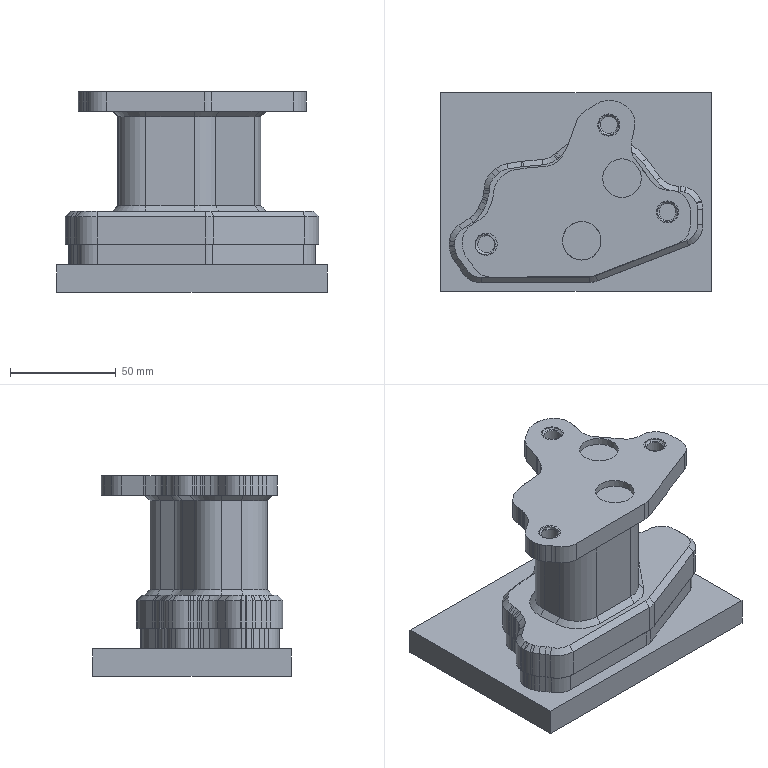NC program | NX | posted by the shop | part box 128.162 x 94.109 x 95 mm
Lines 2106 to 2518 of 2518:
2105 TOOL CALL 15 Z S8000
2106 CALL LBL101
2107 M3 M8
2108 M51
2109 CYCL DEF 32.0 TOLERANCE
2110 CYCL DEF 32.1 T0.012
2111 CYCL DEF 32.2 HSC-MODE:0
2112 L M126
2113 L A+0.0 C+0.0 FMAX
2114 L X-20.1628 Y-49.7703 FMAX
2115 L Z135. FMAX
2116 L Z72.4361 FMAX
2117 L X-17.9996 Y-44.1738 F1000.
2118 L X-55.0175 Y-29.8654
2119 CC X-49.4871 Y-15.5573
2120 C X-64.8269 Y-15.5573 DR-
2121 L Y-8.3845
2122 CC X-49.4871 Y-8.3845
2123 C X-63.8198 Y-2.9181 DR-
2124 L X-63.6526 Y-2.4797
2125 CC X-49.3199 Y-7.9461
2126 C X-53.2724 Y6.8757 DR-
2127 L X-53.2021 Y6.8944
2128 CC X-49.2496 Y-7.9274
2129 C X-49.2496 Y7.4124 DR-
2130 L X-48.4571
2131 CC X-48.4571 Y13.2602
2132 C X-43.7903 Y9.7363 DR+
2133 L X-37.044 Y18.6706
2134 CC X-11.9727 Y-.2607
2135 C X-7.4357 Y30.826 DR-
2136 L X-4.8349 Y30.4464
2137 CC X-9.3718 Y-.6402
2138 C X12.4228 Y21.9862 DR-
2139 CC X16.4797 Y26.1979
2140 C X12.9027 Y21.5717 DR+
2141 L X13.3406 Y21.2331
2142 CC X16.9177 Y25.8593
2143 C X16.4254 Y20.0323 DR+
2144 L X25.5719 Y19.2596
2145 CC X24.2807 Y3.9743
2146 C X26.5942 Y19.1386 DR-
2147 L X33.2783 Y18.1189
2148 CC X30.9648 Y2.9545
2149 C X41.0283 Y14.532 DR-
2150 L X42.9771 Y12.838
2151 CC X32.9137 Y1.2606
2152 C X48.2402 Y1.8989 DR-
2153 CC X54.0829 Y2.1423
2154 C X48.2836 Y1.3906 DR+
2155 L X48.4707 Y-.0522
2156 CC X54.2699 Y.6995
2157 C X48.6732 Y-.9956 DR+
2158 L X49.0076 Y-2.0997
2159 CC X54.6044 Y-.4047
2160 C X49.2541 Y-2.7651 DR+
2161 L X50.5606 Y-5.7266
2162 CC X55.9109 Y-3.3662
2163 C X52.7025 Y-8.2552 DR+
2164 L X57.8907 Y-11.66
2165 CC X49.4744 Y-24.4848
2166 C X64.687 Y-22.513 DR-
2167 L X64.6996 Y-22.6105
2168 CC X49.4871 Y-24.5823
2169 C X64.7942 Y-25.5824 DR-
2170 L X64.7448 Y-26.3385
2171 CC X49.4377 Y-25.3384
2172 C X63.9557 Y-30.2918 DR-
2173 L X63.5699 Y-31.4225
2174 CC X49.0519 Y-26.4691
2175 C X61.1604 Y-35.8868 DR-
2176 L X59.4035 Y-38.1457
2177 CC X64.0194 Y-41.7359
2178 C X58.7617 Y-39.176 DR+
2179 CC X44.9698 Y-32.4609
2180 C X44.905 Y-47.8006 DR-
2181 L X-6.3796 Y-47.5841
2182 CC X-6.3149 Y-32.2444
2183 C X-11.8453 Y-46.5526 DR-
2184 L X-17.9996 Y-44.1738
2185 L X-16.197 Y-39.51
2186 L X-53.2149 Y-25.2017
2187 CC X-49.4871 Y-15.5573
2188 C X-59.8269 Y-15.5573 DR-
2189 L Y-8.3845
2190 CC X-49.4871 Y-8.3845
2191 C X-59.1481 Y-4.6999 DR-
2192 L X-58.9809 Y-4.2615
2193 CC X-49.3199 Y-7.9461
2194 C X-51.984 Y2.0445 DR-
2195 CC X-49.2506 Y-7.9274
2196 C X-49.2496 Y2.4124 DR-
2197 L X-48.4571
2198 CC X-48.4571 Y13.2602
2199 C X-39.8001 Y6.7233 DR+
2200 L X-33.0538 Y15.6576
2201 CC X-11.9727 Y-.2607
2202 C X-8.1578 Y25.8784 DR-
2203 L X-5.5569 Y25.4988
2204 CC X-9.3718 Y-.6402
2205 C X8.9541 Y18.3851 DR-
2206 CC X16.4797 Y26.1979
2207 C X9.8442 Y17.6163 DR+
2208 L X10.2822 Y17.2776
2209 CC X16.9177 Y25.8593
2210 C X16.0046 Y15.05 DR+
2211 L X25.1511 Y14.2774
2212 CC X24.2807 Y3.9743
2213 C X25.8401 Y14.1958 DR-
2214 L X32.5242 Y13.1761
2215 CC X30.9648 Y2.9545
2216 C X37.7481 Y10.7583 DR-
2217 L X39.6969 Y9.0643
2218 CC X32.9137 Y1.2606
2219 C X43.2445 Y1.6908 DR-
2220 CC X54.0829 Y2.1423
2221 C X43.3251 Y.7479 DR+
2222 L X43.5123 Y-.696
2223 CC X54.2699 Y.6995
2224 C X43.8879 Y-2.4449 DR+
2225 L X44.2223 Y-3.5491
2226 CC X54.6044 Y-.4047
2227 C X44.6795 Y-4.7833 DR+
2228 L X45.9865 Y-7.7457
2229 CC X55.9109 Y-3.3662
2230 C X49.9592 Y-12.4354 DR+
2231 L X55.1474 Y-15.8402
2232 CC X49.4749 Y-24.4851
2233 C X59.7411 Y-23.2532 DR-
2234 CC X49.4871 Y-24.5823
2235 C X59.8049 Y-25.2564 DR-
2236 L X59.7555 Y-26.0125
2237 CC X49.4377 Y-25.3384
2238 C X59.2235 Y-28.6772 DR-
2239 L X58.8378 Y-29.8079
2240 CC X49.0519 Y-26.4691
2241 C X57.2136 Y-32.8171 DR-
2242 L X55.4567 Y-35.076
2243 CC X64.0194 Y-41.7359
2244 C X54.2662 Y-36.9872 DR+
2245 CC X44.9698 Y-32.4609
2246 C X44.9261 Y-42.8006 DR-
2247 L X-6.3585 Y-42.5841
2248 CC X-6.3149 Y-32.2444
2249 C X-10.0427 Y-41.8888 DR-
2250 L X-16.197 Y-39.51
2251 L X-14.3943 Y-34.8463
2252 L X-51.4122 Y-20.538
2253 CC X-49.4871 Y-15.5573
2254 C X-54.8269 Y-15.5573 DR-
2255 L Y-8.3845
2256 CC X-49.4871 Y-8.3845
2257 C X-54.4763 Y-6.4816 DR-
2258 L X-54.3091 Y-6.0433
2259 CC X-49.3199 Y-7.9461
2260 C X-50.679 Y-2.7822 DR-
2261 CC X-49.2507 Y-7.9274
2262 C X-49.2501 Y-2.5876 DR-
2263 L X-48.4571
2264 CC X-48.4571 Y13.2602
2265 C X-35.8099 Y3.7103 DR+
2266 L X-29.0636 Y12.6446
2267 CC X-11.9727 Y-.2607
2268 C X-8.8799 Y20.9308 DR-
2269 L X-6.279 Y20.5513
2270 CC X-9.3718 Y-.6402
2271 C X5.4854 Y14.784 DR-
2272 CC X16.4797 Y26.1979
2273 C X6.7858 Y13.6608 DR+
2274 L X7.2237 Y13.3221
2275 CC X16.9177 Y25.8593
2276 C X15.5837 Y10.0677 DR+
2277 L X24.7302 Y9.2951
2278 CC X24.2807 Y3.9743
2279 C X25.086 Y9.253 DR-
2280 L X31.7702 Y8.2333
2281 CC X30.9648 Y2.9545
2282 C X34.4679 Y6.9847 DR-
2283 L X36.4168 Y5.2907
2284 CC X32.9137 Y1.2606
2285 C X38.2489 Y1.4828 DR-
2286 CC X54.0829 Y2.1423
2287 C X38.3666 Y.1052 DR+
2288 L X38.5538 Y-1.3392
2289 CC X54.2699 Y.6995
2290 C X39.1025 Y-3.8942 DR+
2291 L X39.4369 Y-4.9984
2292 CC X54.6044 Y-.4047
2293 C X40.1049 Y-6.8015 DR+
2294 L X41.4121 Y-9.7643
2295 CC X55.9109 Y-3.3662
2296 C X47.2159 Y-16.6157 DR+
2297 L X52.4044 Y-20.0206
2298 CC X49.475 Y-24.4852
2299 C X54.7795 Y-23.8724 DR-
2300 CC X49.4871 Y-24.582
2301 C X54.8155 Y-24.9304 DR-
2302 L X54.7661 Y-25.6865
2303 CC X49.4377 Y-25.3384
2304 C X54.4914 Y-27.0627 DR-
2305 L X54.1056 Y-28.1933
2306 CC X49.0519 Y-26.4691
2307 C X53.2669 Y-29.7474 DR-
2308 L X51.5099 Y-32.0063
2309 CC X64.0194 Y-41.7359
2310 C X49.7708 Y-34.7984 DR+
2311 CC X44.9698 Y-32.4609
2312 C X44.9473 Y-37.8006 DR-
2313 L X-6.3374 Y-37.5842
2314 CC X-6.3149 Y-32.2444
2315 C X-8.24 Y-37.2251 DR-
2316 L X-14.3943 Y-34.8463
2317 L X-12.5917 Y-30.1826
2318 L X-49.6096 Y-15.8742
2319 CC X-49.4871 Y-15.5573
2320 C X-49.8269 Y-15.5573 DR-
2321 L Y-8.3845
2322 CC X-49.4871 Y-8.3845
2323 C X-49.8046 Y-8.2634 DR-
2324 L X-49.6373 Y-7.825
2325 CC X-49.3192 Y-7.9443
2326 C X-49.3739 Y-7.609 DR-
2327 L X-49.3416 Y-7.6
2328 CC X-49.2507 Y-7.9274
2329 C X-49.2507 Y-7.5876 DR-
2330 L X-48.4571
2331 CC X-48.4571 Y13.2602
2332 C X-31.8196 Y.6973 DR+
2333 L X-25.0734 Y9.6316
2334 CC X-11.9727 Y-.2607
2335 C X-9.602 Y15.9832 DR-
2336 L X-7.0011 Y15.6037
2337 CC X-9.3718 Y-.6402
2338 C X2.0167 Y11.1829 DR-
2339 CC X16.4797 Y26.1979
2340 C X3.7274 Y9.7053 DR+
2341 L X4.1653 Y9.3666
2342 CC X16.9177 Y25.8593
2343 C X15.1628 Y5.0855 DR+
2344 L X24.332 Y4.3102
2345 L X31.0161 Y3.2904
2346 CC X30.9648 Y2.9545
2347 C X31.1878 Y3.211 DR-
2348 L X33.1366 Y1.517
2349 CC X32.9137 Y1.2606
2350 C X33.2532 Y1.2747 DR-
2351 CC X54.0829 Y2.1423
2352 C X33.4081 Y-.5375 DR+
2353 L X33.5954 Y-1.9824
2354 CC X54.2699 Y.6995
2355 C X34.3172 Y-5.3435 DR+
2356 L X34.6516 Y-6.4477
2357 CC X54.6044 Y-.4047
2358 C X35.5303 Y-8.8197 DR+
2359 L X36.8377 Y-11.783
2360 CC X55.9109 Y-3.3662
2361 C X44.4726 Y-20.7959 DR+
2362 L X49.6614 Y-24.2011
2363 CC X49.475 Y-24.4852
2364 C X49.8125 Y-24.4462 DR-
2365 L X49.8178 Y-24.4916
2366 L X49.8239 Y-24.5369
2367 CC X49.4871 Y-24.582
2368 C X49.8262 Y-24.6042 DR-
2369 L X49.7767 Y-25.3605
2370 CC X49.4377 Y-25.3384
2371 C X49.7593 Y-25.4481 DR-
2372 L X49.3735 Y-26.5788
2373 CC X49.0519 Y-26.4691
2374 C X49.3201 Y-26.6777 DR-
2375 L X47.5632 Y-28.9366
2376 CC X64.0194 Y-41.7359
2377 C X45.2753 Y-32.6096 DR+
2378 CC X44.9698 Y-32.4609
2379 C X44.9684 Y-32.8007 DR-
2380 L X-6.3163 Y-32.5842
2381 CC X-6.3149 Y-32.2444
2382 C X-6.4374 Y-32.5614 DR-
2383 L X-12.5917 Y-30.1826
2384 L X-10.789 Y-25.5188
2385 L X-44.8269 Y-12.3624
2386 L Y-12.3314
2387 CC X-48.4571 Y13.2602
2388 C X-27.8294 Y-2.3157 DR+
2389 L X-21.0831 Y6.6186
2390 CC X-11.9727 Y-.2607
2391 C X-10.324 Y11.0357 DR-
2392 L X-7.7232 Y10.6561
2393 CC X-9.3718 Y-.6402
2394 C X-1.452 Y7.5818 DR-
2395 CC X16.4797 Y26.1979
2396 C X.6689 Y5.7498 DR+
2397 L X1.1068 Y5.4112
2398 CC X16.9177 Y25.8593
2399 C X14.7415 Y.1033 DR+
2400 L X23.7436 Y-.6579
2401 L X28.4754 Y-1.3798
2402 L X28.6369 Y-2.6257
2403 CC X54.2699 Y.6995
2404 C X29.5318 Y-6.7929 DR+
2405 L X29.8663 Y-7.897
2406 CC X54.6044 Y-.4047
2407 C X30.9557 Y-10.8379 DR+
2408 L X32.2633 Y-13.8016
2409 CC X55.9109 Y-3.3662
2410 C X41.7293 Y-24.9762 DR+
2411 L X43.4388 Y-26.098
2412 CC X64.0194 Y-41.7359
2413 C X42.2571 Y-27.7892 DR+
2414 L X-5.4361 Y-27.5879
2415 L X-10.789 Y-25.5188
2416 L X-8.9864 Y-20.8551
2417 L X-31.1624 Y-12.2835
2418 CC X-48.4571 Y13.2602
2419 C X-23.8392 Y-5.3287 DR+
2420 L X-17.0929 Y3.6056
2421 CC X-11.9727 Y-.2607
2422 C X-11.0461 Y6.0881 DR-
2423 L X-8.4453 Y5.7085
2424 CC X-9.3718 Y-.6402
2425 C X-4.9208 Y3.9807 DR-
2426 CC X16.4797 Y26.1979
2427 C X-2.3895 Y1.7943 DR+
2428 L X-1.9516 Y1.4557
2429 CC X16.9177 Y25.8593
2430 C X14.3202 Y-4.8789 DR+
2431 L X23.1553 Y-5.626
2432 L X24.1085 Y-5.7714
2433 CC X54.2699 Y.6995
2434 C X24.7465 Y-8.2422 DR+
2435 L X25.0809 Y-9.3463
2436 CC X54.6044 Y-.4047
2437 C X26.3812 Y-12.8561 DR+
2438 L X27.6889 Y-15.8202
2439 CC X55.9109 Y-3.3662
2440 C X31.9103 Y-22.7455 DR+
2441 L X-4.4932 Y-22.5918
2442 L X-8.9864 Y-20.8551
2443 L X-7.1837 Y-16.1914
2444 L X-21.6896 Y-10.5845
2445 CC X-48.4571 Y13.2602
2446 C X-19.849 Y-8.3417 DR+
2447 L X-13.1027 Y.5926
2448 CC X-11.9727 Y-.2607
2449 C X-11.7682 Y1.1405 DR-
2450 L X-9.1673 Y.7609
2451 CC X-9.3718 Y-.6402
2452 C X-8.3895 Y.3796 DR-
2453 CC X16.4797 Y26.1979
2454 C X-5.448 Y-2.1612 DR+
2455 L X-5.01 Y-2.4998
2456 CC X16.9177 Y25.8593
2457 C X13.899 Y-9.8612 DR+
2458 L X20.1732 Y-10.3917
2459 L X20.2956 Y-10.7957
2460 CC X54.6044 Y-.4047
2461 C X21.8066 Y-14.8743 DR+
2462 L X23.0568 Y-17.7081
2463 L X-3.5503 Y-17.5957
2464 L X-7.1837 Y-16.1914
2465 L X-5.3811 Y-11.5276
2466 L X-13.5927 Y-8.3536
2467 L X-10.597 Y-4.3863
2468 CC X16.4797 Y26.1979
2469 C X-8.5064 Y-6.1167 DR+
2470 L X-8.0685 Y-6.4553
2471 CC X16.9177 Y25.8593
2472 C X3.2226 Y-12.6243 DR+
2473 L X-2.6075 Y-12.5997
2474 L X-5.3811 Y-11.5276
2475 L X-7.5442 Y-17.1241
2476 L Z135. FMAX
2477 PLANE RESET STAY
2478 M50
2479 M5
2480 M9
2481 CALL LBL100
2482 M30
2483 ;
2484 LBL100
2485 M129
2486 M140 MB MAX
2487 L X-1.0 R0 FMAX M91
2488 L Y-1.0 R0 FMAX M91
2489 L A0.0 C0.0 FMAX
2490 PLANE RESET STAY
2491 CYCL DEF 7.0 DATUM SHIFT
2492 CYCL DEF 7.1 X+0.
2493 CYCL DEF 7.2 Y+0.
2494 CYCL DEF 7.3 Z+0.
2495 CYCL DEF 32.0 TOLERANCE
2496 CYCL DEF 32.1
2497 CYCL DEF 32.2
2498 LBL0
2499 ;
2500 ;
2501 LBL101
2502 M129
2503 M140 MB MAX
2504 L X-1.0 R0 FMAX M91
2505 L Y-600.0 R0 FMAX M91
2506 L A0.0 C0.0 FMAX
2507 PLANE RESET STAY
2508 CYCL DEF 7.0 DATUM SHIFT
2509 CYCL DEF 7.1 X+0.
2510 CYCL DEF 7.2 Y+0.
2511 CYCL DEF 7.3 Z+0.
2512 CYCL DEF 32.0 TOLERANCE
2513 CYCL DEF 32.1
2514 CYCL DEF 32.2
2515 LBL0
2516 ;
2517 END PGM B MM